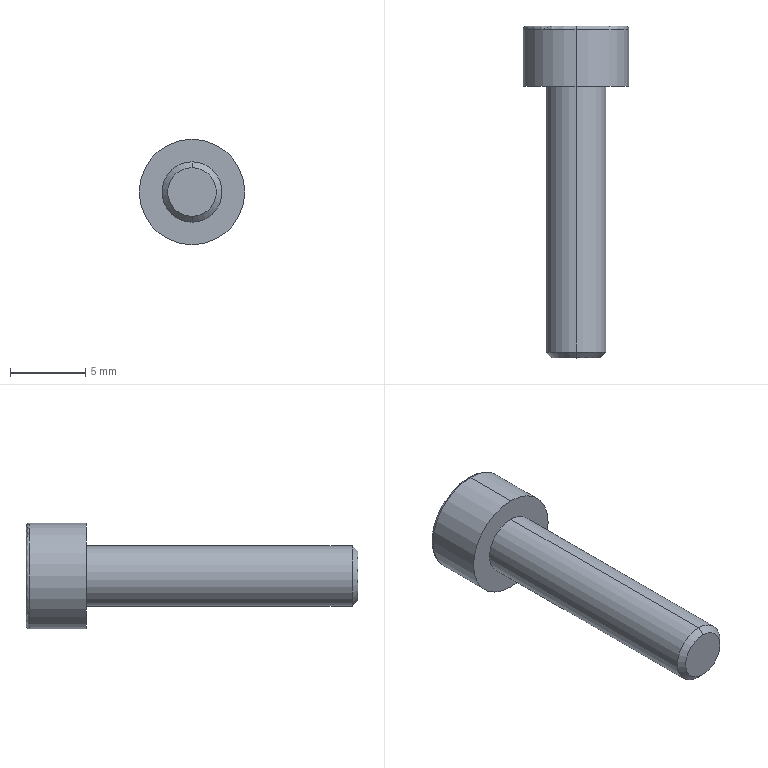Part | SolidWorks | features ICE 2, Chamfer 1, Extrusion 1, Fillet 1, RefAxis 1 | 1 solid | 18 faces | box 7 x 22 x 7 mm | volume 362.728 mm3 | plane 10 | cylinder 4 | cone 2 | torus 2 | commonest cylinder face diameters 4 x2 7 x2
STEP:
#1=CARTESIAN_POINT('',(0.,-18.,-1.61));
#2=VERTEX_POINT('',#1);
#3=CARTESIAN_POINT('',(0.,-18.,1.61));
#4=VERTEX_POINT('',#3);
#5=CARTESIAN_POINT('',(0.,-18.,0.));
#6=DIRECTION('',(0.,-1.,0.));
#7=DIRECTION('',(0.,0.,-1.));
#8=AXIS2_PLACEMENT_3D('',#5,#6,#7);
#9=CIRCLE('',#8,1.61);
#10=EDGE_CURVE('',#2,#4,#9,.T.);
#11=ORIENTED_EDGE('',*,*,#10,.F.);
#12=CARTESIAN_POINT('',(0.,-17.61,-2.));
#13=VERTEX_POINT('',#12);
#14=CARTESIAN_POINT('',(0.,-18.,-1.61));
#15=DIRECTION('',(0.,0.7071,-0.7071));
#16=VECTOR('',#15,1000.);
#17=LINE('',#14,#16);
#18=EDGE_CURVE('',#2,#13,#17,.T.);
#19=ORIENTED_EDGE('',*,*,#18,.T.);
#20=CARTESIAN_POINT('',(0.,-17.61,2.));
#21=VERTEX_POINT('',#20);
#22=CARTESIAN_POINT('',(0.,-17.61,0.));
#23=DIRECTION('',(0.,1.,0.));
#24=DIRECTION('',(0.,0.,-1.));
#25=AXIS2_PLACEMENT_3D('',#22,#23,#24);
#26=CIRCLE('',#25,2.);
#27=EDGE_CURVE('',#21,#13,#26,.T.);
#28=ORIENTED_EDGE('',*,*,#27,.F.);
#29=CARTESIAN_POINT('',(0.,-18.,1.61));
#30=DIRECTION('',(0.,0.7071,0.7071));
#31=VECTOR('',#30,1000.);
#32=LINE('',#29,#31);
#33=EDGE_CURVE('',#4,#21,#32,.T.);
#34=ORIENTED_EDGE('',*,*,#33,.F.);
#35=EDGE_LOOP('',(#11,#19,#28,#34));
#36=FACE_OUTER_BOUND('',#35,.T.);
#37=CARTESIAN_POINT('',(0.,-18.,0.));
#38=DIRECTION('',(0.,1.,0.));
#39=DIRECTION('',(0.,0.,1.));
#40=AXIS2_PLACEMENT_3D('',#37,#38,#39);
#41=CONICAL_SURFACE('',#40,1.61,0.7854);
#42=ADVANCED_FACE('',(#36),#41,.T.);
#43=ORIENTED_EDGE('',*,*,#27,.T.);
#44=CARTESIAN_POINT('',(0.,0.,-2.));
#45=VERTEX_POINT('',#44);
#46=CARTESIAN_POINT('',(0.,-18.,-2.));
#47=DIRECTION('',(0.,1.,0.));
#48=VECTOR('',#47,1000.);
#49=LINE('',#46,#48);
#50=EDGE_CURVE('',#13,#45,#49,.T.);
#51=ORIENTED_EDGE('',*,*,#50,.T.);
#52=CARTESIAN_POINT('',(0.,0.,2.));
#53=VERTEX_POINT('',#52);
#54=CARTESIAN_POINT('',(0.,0.,0.));
#55=DIRECTION('',(0.,-1.,0.));
#56=DIRECTION('',(0.,0.,1.));
#57=AXIS2_PLACEMENT_3D('',#54,#55,#56);
#58=CIRCLE('',#57,2.);
#59=EDGE_CURVE('',#45,#53,#58,.T.);
#60=ORIENTED_EDGE('',*,*,#59,.T.);
#61=CARTESIAN_POINT('',(0.,-18.,2.));
#62=DIRECTION('',(0.,1.,0.));
#63=VECTOR('',#62,1000.);
#64=LINE('',#61,#63);
#65=EDGE_CURVE('',#21,#53,#64,.T.);
#66=ORIENTED_EDGE('',*,*,#65,.F.);
#67=EDGE_LOOP('',(#43,#51,#60,#66));
#68=FACE_OUTER_BOUND('',#67,.T.);
#69=CARTESIAN_POINT('',(0.,-18.,0.));
#70=DIRECTION('',(0.,1.,0.));
#71=DIRECTION('',(0.,0.,1.));
#72=AXIS2_PLACEMENT_3D('',#69,#70,#71);
#73=CYLINDRICAL_SURFACE('',#72,2.);
#74=ADVANCED_FACE('',(#68),#73,.T.);
#75=CARTESIAN_POINT('',(0.,3.8,-3.5));
#76=VERTEX_POINT('',#75);
#77=CARTESIAN_POINT('',(0.,3.8,3.5));
#78=VERTEX_POINT('',#77);
#79=CARTESIAN_POINT('',(0.,3.8,0.));
#80=DIRECTION('',(0.,-1.,0.));
#81=DIRECTION('',(0.,0.,1.));
#82=AXIS2_PLACEMENT_3D('',#79,#80,#81);
#83=CIRCLE('',#82,3.5);
#84=EDGE_CURVE('',#76,#78,#83,.T.);
#85=ORIENTED_EDGE('',*,*,#84,.F.);
#86=CARTESIAN_POINT('',(0.,4.,-3.3));
#87=VERTEX_POINT('',#86);
#88=CARTESIAN_POINT('',(0.,3.8,-3.3));
#89=DIRECTION('',(1.,0.,0.));
#90=DIRECTION('',(0.,0.,-1.));
#91=AXIS2_PLACEMENT_3D('',#88,#89,#90);
#92=CIRCLE('',#91,0.2);
#93=EDGE_CURVE('',#76,#87,#92,.T.);
#94=ORIENTED_EDGE('',*,*,#93,.T.);
#95=CARTESIAN_POINT('',(0.,4.,3.3));
#96=VERTEX_POINT('',#95);
#97=CARTESIAN_POINT('',(0.,4.,0.));
#98=DIRECTION('',(0.,1.,0.));
#99=DIRECTION('',(0.,0.,1.));
#100=AXIS2_PLACEMENT_3D('',#97,#98,#99);
#101=CIRCLE('',#100,3.3);
#102=EDGE_CURVE('',#96,#87,#101,.T.);
#103=ORIENTED_EDGE('',*,*,#102,.F.);
#104=CARTESIAN_POINT('',(0.,3.8,3.3));
#105=DIRECTION('',(-1.,0.,0.));
#106=DIRECTION('',(0.,0.,1.));
#107=AXIS2_PLACEMENT_3D('',#104,#105,#106);
#108=CIRCLE('',#107,0.2);
#109=EDGE_CURVE('',#78,#96,#108,.T.);
#110=ORIENTED_EDGE('',*,*,#109,.F.);
#111=EDGE_LOOP('',(#85,#94,#103,#110));
#112=FACE_OUTER_BOUND('',#111,.T.);
#113=CARTESIAN_POINT('',(0.,3.8,0.));
#114=DIRECTION('',(0.,1.,0.));
#115=DIRECTION('',(0.,0.,1.));
#116=AXIS2_PLACEMENT_3D('',#113,#114,#115);
#117=TOROIDAL_SURFACE('',#116,3.3,0.2);
#118=ADVANCED_FACE('',(#112),#117,.T.);
#119=ORIENTED_EDGE('',*,*,#84,.T.);
#120=CARTESIAN_POINT('',(0.,0.,3.5));
#121=VERTEX_POINT('',#120);
#122=CARTESIAN_POINT('',(0.,4.,3.5));
#123=DIRECTION('',(0.,-1.,0.));
#124=VECTOR('',#123,1000.);
#125=LINE('',#122,#124);
#126=EDGE_CURVE('',#78,#121,#125,.T.);
#127=ORIENTED_EDGE('',*,*,#126,.T.);
#128=CARTESIAN_POINT('',(0.,0.,-3.5));
#129=VERTEX_POINT('',#128);
#130=CARTESIAN_POINT('',(0.,0.,0.));
#131=DIRECTION('',(0.,1.,0.));
#132=DIRECTION('',(0.,0.,1.));
#133=AXIS2_PLACEMENT_3D('',#130,#131,#132);
#134=CIRCLE('',#133,3.5);
#135=EDGE_CURVE('',#121,#129,#134,.T.);
#136=ORIENTED_EDGE('',*,*,#135,.T.);
#137=CARTESIAN_POINT('',(0.,4.,-3.5));
#138=DIRECTION('',(0.,-1.,0.));
#139=VECTOR('',#138,1000.);
#140=LINE('',#137,#139);
#141=EDGE_CURVE('',#76,#129,#140,.T.);
#142=ORIENTED_EDGE('',*,*,#141,.F.);
#143=EDGE_LOOP('',(#119,#127,#136,#142));
#144=FACE_OUTER_BOUND('',#143,.T.);
#145=CARTESIAN_POINT('',(0.,4.,0.));
#146=DIRECTION('',(0.,-1.,0.));
#147=DIRECTION('',(0.,0.,-1.));
#148=AXIS2_PLACEMENT_3D('',#145,#146,#147);
#149=CYLINDRICAL_SURFACE('',#148,3.5);
#150=ADVANCED_FACE('',(#144),#149,.T.);
#151=CARTESIAN_POINT('',(0.,0.,0.));
#152=DIRECTION('',(0.,1.,0.));
#153=DIRECTION('',(0.,0.,1.));
#154=AXIS2_PLACEMENT_3D('',#151,#152,#153);
#155=CIRCLE('',#154,3.5);
#156=EDGE_CURVE('',#129,#121,#155,.T.);
#157=ORIENTED_EDGE('',*,*,#156,.F.);
#158=ORIENTED_EDGE('',*,*,#135,.F.);
#159=EDGE_LOOP('',(#157,#158));
#160=FACE_OUTER_BOUND('',#159,.T.);
#161=CARTESIAN_POINT('',(0.,0.,0.));
#162=DIRECTION('',(0.,-1.,0.));
#163=DIRECTION('',(0.,0.,1.));
#164=AXIS2_PLACEMENT_3D('',#161,#162,#163);
#165=CIRCLE('',#164,2.);
#166=EDGE_CURVE('',#53,#45,#165,.T.);
#167=ORIENTED_EDGE('',*,*,#166,.F.);
#168=ORIENTED_EDGE('',*,*,#59,.F.);
#169=EDGE_LOOP('',(#167,#168));
#170=FACE_BOUND('',#169,.T.);
#171=CARTESIAN_POINT('',(0.,0.,0.));
#172=DIRECTION('',(0.,1.,0.));
#173=DIRECTION('',(0.,0.,1.));
#174=AXIS2_PLACEMENT_3D('',#171,#172,#173);
#175=PLANE('',#174);
#176=ADVANCED_FACE('',(#160,#170),#175,.F.);
#177=ORIENTED_EDGE('',*,*,#126,.F.);
#178=CARTESIAN_POINT('',(0.,3.8,0.));
#179=DIRECTION('',(0.,-1.,0.));
#180=DIRECTION('',(0.,0.,1.));
#181=AXIS2_PLACEMENT_3D('',#178,#179,#180);
#182=CIRCLE('',#181,3.5);
#183=EDGE_CURVE('',#78,#76,#182,.T.);
#184=ORIENTED_EDGE('',*,*,#183,.T.);
#185=ORIENTED_EDGE('',*,*,#141,.T.);
#186=ORIENTED_EDGE('',*,*,#156,.T.);
#187=EDGE_LOOP('',(#177,#184,#185,#186));
#188=FACE_OUTER_BOUND('',#187,.T.);
#189=CARTESIAN_POINT('',(0.,4.,0.));
#190=DIRECTION('',(0.,-1.,0.));
#191=DIRECTION('',(0.,0.,-1.));
#192=AXIS2_PLACEMENT_3D('',#189,#190,#191);
#193=CYLINDRICAL_SURFACE('',#192,3.5);
#194=ADVANCED_FACE('',(#188),#193,.T.);
#195=ORIENTED_EDGE('',*,*,#102,.T.);
#196=CARTESIAN_POINT('',(0.,4.,0.));
#197=DIRECTION('',(0.,1.,0.));
#198=DIRECTION('',(0.,0.,1.));
#199=AXIS2_PLACEMENT_3D('',#196,#197,#198);
#200=CIRCLE('',#199,3.3);
#201=EDGE_CURVE('',#87,#96,#200,.T.);
#202=ORIENTED_EDGE('',*,*,#201,.T.);
#203=EDGE_LOOP('',(#195,#202));
#204=FACE_OUTER_BOUND('',#203,.T.);
#205=CARTESIAN_POINT('',(0.8862,4.,1.535));
#206=VERTEX_POINT('',#205);
#207=CARTESIAN_POINT('',(1.772,4.,0.));
#208=VERTEX_POINT('',#207);
#209=CARTESIAN_POINT('',(0.8862,4.,1.535));
#210=DIRECTION('',(0.5,0.,-0.866));
#211=VECTOR('',#210,1000.);
#212=LINE('',#209,#211);
#213=EDGE_CURVE('',#206,#208,#212,.T.);
#214=ORIENTED_EDGE('',*,*,#213,.F.);
#215=CARTESIAN_POINT('',(-0.8862,4.,1.535));
#216=VERTEX_POINT('',#215);
#217=CARTESIAN_POINT('',(-0.8862,4.,1.535));
#218=DIRECTION('',(1.,0.,0.));
#219=VECTOR('',#218,1000.);
#220=LINE('',#217,#219);
#221=EDGE_CURVE('',#216,#206,#220,.T.);
#222=ORIENTED_EDGE('',*,*,#221,.F.);
#223=CARTESIAN_POINT('',(-1.772,4.,0.));
#224=VERTEX_POINT('',#223);
#225=CARTESIAN_POINT('',(-1.772,4.,0.));
#226=DIRECTION('',(0.5,0.,0.866));
#227=VECTOR('',#226,1000.);
#228=LINE('',#225,#227);
#229=EDGE_CURVE('',#224,#216,#228,.T.);
#230=ORIENTED_EDGE('',*,*,#229,.F.);
#231=CARTESIAN_POINT('',(-0.8862,4.,-1.535));
#232=VERTEX_POINT('',#231);
#233=CARTESIAN_POINT('',(-0.8862,4.,-1.535));
#234=DIRECTION('',(-0.5,0.,0.866));
#235=VECTOR('',#234,1000.);
#236=LINE('',#233,#235);
#237=EDGE_CURVE('',#232,#224,#236,.T.);
#238=ORIENTED_EDGE('',*,*,#237,.F.);
#239=CARTESIAN_POINT('',(0.8862,4.,-1.535));
#240=VERTEX_POINT('',#239);
#241=CARTESIAN_POINT('',(0.8862,4.,-1.535));
#242=DIRECTION('',(-1.,0.,0.));
#243=VECTOR('',#242,1000.);
#244=LINE('',#241,#243);
#245=EDGE_CURVE('',#240,#232,#244,.T.);
#246=ORIENTED_EDGE('',*,*,#245,.F.);
#247=CARTESIAN_POINT('',(1.772,4.,0.));
#248=DIRECTION('',(-0.5,0.,-0.866));
#249=VECTOR('',#248,1000.);
#250=LINE('',#247,#249);
#251=EDGE_CURVE('',#208,#240,#250,.T.);
#252=ORIENTED_EDGE('',*,*,#251,.F.);
#253=EDGE_LOOP('',(#214,#222,#230,#238,#246,#252));
#254=FACE_BOUND('',#253,.T.);
#255=CARTESIAN_POINT('',(0.,4.,0.));
#256=DIRECTION('',(0.,1.,0.));
#257=DIRECTION('',(0.,0.,1.));
#258=AXIS2_PLACEMENT_3D('',#255,#256,#257);
#259=PLANE('',#258);
#260=ADVANCED_FACE('',(#204,#254),#259,.T.);
#261=ORIENTED_EDGE('',*,*,#213,.T.);
#262=CARTESIAN_POINT('',(1.772,2.,0.));
#263=VERTEX_POINT('',#262);
#264=CARTESIAN_POINT('',(1.772,2.,0.));
#265=DIRECTION('',(0.,1.,0.));
#266=VECTOR('',#265,1000.);
#267=LINE('',#264,#266);
#268=EDGE_CURVE('',#263,#208,#267,.T.);
#269=ORIENTED_EDGE('',*,*,#268,.F.);
#270=CARTESIAN_POINT('',(0.8862,2.,1.535));
#271=VERTEX_POINT('',#270);
#272=CARTESIAN_POINT('',(0.8862,2.,1.535));
#273=DIRECTION('',(0.5,0.,-0.866));
#274=VECTOR('',#273,1000.);
#275=LINE('',#272,#274);
#276=EDGE_CURVE('',#271,#263,#275,.T.);
#277=ORIENTED_EDGE('',*,*,#276,.F.);
#278=CARTESIAN_POINT('',(0.8862,2.,1.535));
#279=DIRECTION('',(0.,1.,0.));
#280=VECTOR('',#279,1000.);
#281=LINE('',#278,#280);
#282=EDGE_CURVE('',#271,#206,#281,.T.);
#283=ORIENTED_EDGE('',*,*,#282,.T.);
#284=EDGE_LOOP('',(#261,#269,#277,#283));
#285=FACE_OUTER_BOUND('',#284,.T.);
#286=CARTESIAN_POINT('',(0.8862,2.,1.535));
#287=DIRECTION('',(0.866,0.,0.5));
#288=DIRECTION('',(0.5,0.,-0.866));
#289=AXIS2_PLACEMENT_3D('',#286,#287,#288);
#290=PLANE('',#289);
#291=ADVANCED_FACE('',(#285),#290,.F.);
#292=ORIENTED_EDGE('',*,*,#221,.T.);
#293=ORIENTED_EDGE('',*,*,#282,.F.);
#294=CARTESIAN_POINT('',(-0.8862,2.,1.535));
#295=VERTEX_POINT('',#294);
#296=CARTESIAN_POINT('',(-0.8862,2.,1.535));
#297=DIRECTION('',(1.,0.,0.));
#298=VECTOR('',#297,1000.);
#299=LINE('',#296,#298);
#300=EDGE_CURVE('',#295,#271,#299,.T.);
#301=ORIENTED_EDGE('',*,*,#300,.F.);
#302=CARTESIAN_POINT('',(-0.8862,2.,1.535));
#303=DIRECTION('',(0.,1.,0.));
#304=VECTOR('',#303,1000.);
#305=LINE('',#302,#304);
#306=EDGE_CURVE('',#295,#216,#305,.T.);
#307=ORIENTED_EDGE('',*,*,#306,.T.);
#308=EDGE_LOOP('',(#292,#293,#301,#307));
#309=FACE_OUTER_BOUND('',#308,.T.);
#310=CARTESIAN_POINT('',(-0.8862,2.,1.535));
#311=DIRECTION('',(0.,0.,1.));
#312=DIRECTION('',(1.,0.,0.));
#313=AXIS2_PLACEMENT_3D('',#310,#311,#312);
#314=PLANE('',#313);
#315=ADVANCED_FACE('',(#309),#314,.F.);
#316=ORIENTED_EDGE('',*,*,#229,.T.);
#317=ORIENTED_EDGE('',*,*,#306,.F.);
#318=CARTESIAN_POINT('',(-1.772,2.,0.));
#319=VERTEX_POINT('',#318);
#320=CARTESIAN_POINT('',(-1.772,2.,0.));
#321=DIRECTION('',(0.5,0.,0.866));
#322=VECTOR('',#321,1000.);
#323=LINE('',#320,#322);
#324=EDGE_CURVE('',#319,#295,#323,.T.);
#325=ORIENTED_EDGE('',*,*,#324,.F.);
#326=CARTESIAN_POINT('',(-1.772,2.,0.));
#327=DIRECTION('',(0.,1.,0.));
#328=VECTOR('',#327,1000.);
#329=LINE('',#326,#328);
#330=EDGE_CURVE('',#319,#224,#329,.T.);
#331=ORIENTED_EDGE('',*,*,#330,.T.);
#332=EDGE_LOOP('',(#316,#317,#325,#331));
#333=FACE_OUTER_BOUND('',#332,.T.);
#334=CARTESIAN_POINT('',(-1.772,2.,0.));
#335=DIRECTION('',(-0.866,0.,0.5));
#336=DIRECTION('',(0.5,0.,0.866));
#337=AXIS2_PLACEMENT_3D('',#334,#335,#336);
#338=PLANE('',#337);
#339=ADVANCED_FACE('',(#333),#338,.F.);
#340=ORIENTED_EDGE('',*,*,#237,.T.);
#341=ORIENTED_EDGE('',*,*,#330,.F.);
#342=CARTESIAN_POINT('',(-0.8862,2.,-1.535));
#343=VERTEX_POINT('',#342);
#344=CARTESIAN_POINT('',(-0.8862,2.,-1.535));
#345=DIRECTION('',(-0.5,0.,0.866));
#346=VECTOR('',#345,1000.);
#347=LINE('',#344,#346);
#348=EDGE_CURVE('',#343,#319,#347,.T.);
#349=ORIENTED_EDGE('',*,*,#348,.F.);
#350=CARTESIAN_POINT('',(-0.8862,2.,-1.535));
#351=DIRECTION('',(0.,1.,0.));
#352=VECTOR('',#351,1000.);
#353=LINE('',#350,#352);
#354=EDGE_CURVE('',#343,#232,#353,.T.);
#355=ORIENTED_EDGE('',*,*,#354,.T.);
#356=EDGE_LOOP('',(#340,#341,#349,#355));
#357=FACE_OUTER_BOUND('',#356,.T.);
#358=CARTESIAN_POINT('',(-0.8862,2.,-1.535));
#359=DIRECTION('',(-0.866,0.,-0.5));
#360=DIRECTION('',(-0.5,0.,0.866));
#361=AXIS2_PLACEMENT_3D('',#358,#359,#360);
#362=PLANE('',#361);
#363=ADVANCED_FACE('',(#357),#362,.F.);
#364=ORIENTED_EDGE('',*,*,#245,.T.);
#365=ORIENTED_EDGE('',*,*,#354,.F.);
#366=CARTESIAN_POINT('',(0.8862,2.,-1.535));
#367=VERTEX_POINT('',#366);
#368=CARTESIAN_POINT('',(0.8862,2.,-1.535));
#369=DIRECTION('',(-1.,0.,0.));
#370=VECTOR('',#369,1000.);
#371=LINE('',#368,#370);
#372=EDGE_CURVE('',#367,#343,#371,.T.);
#373=ORIENTED_EDGE('',*,*,#372,.F.);
#374=CARTESIAN_POINT('',(0.8862,2.,-1.535));
#375=DIRECTION('',(0.,1.,0.));
#376=VECTOR('',#375,1000.);
#377=LINE('',#374,#376);
#378=EDGE_CURVE('',#367,#240,#377,.T.);
#379=ORIENTED_EDGE('',*,*,#378,.T.);
#380=EDGE_LOOP('',(#364,#365,#373,#379));
#381=FACE_OUTER_BOUND('',#380,.T.);
#382=CARTESIAN_POINT('',(0.8862,2.,-1.535));
#383=DIRECTION('',(0.,0.,-1.));
#384=DIRECTION('',(-1.,0.,0.));
#385=AXIS2_PLACEMENT_3D('',#382,#383,#384);
#386=PLANE('',#385);
#387=ADVANCED_FACE('',(#381),#386,.F.);
#388=ORIENTED_EDGE('',*,*,#251,.T.);
#389=ORIENTED_EDGE('',*,*,#378,.F.);
#390=CARTESIAN_POINT('',(1.772,2.,0.));
#391=DIRECTION('',(-0.5,0.,-0.866));
#392=VECTOR('',#391,1000.);
#393=LINE('',#390,#392);
#394=EDGE_CURVE('',#263,#367,#393,.T.);
#395=ORIENTED_EDGE('',*,*,#394,.F.);
#396=ORIENTED_EDGE('',*,*,#268,.T.);
#397=EDGE_LOOP('',(#388,#389,#395,#396));
#398=FACE_OUTER_BOUND('',#397,.T.);
#399=CARTESIAN_POINT('',(1.772,2.,0.));
#400=DIRECTION('',(0.866,0.,-0.5));
#401=DIRECTION('',(-0.5,0.,-0.866));
#402=AXIS2_PLACEMENT_3D('',#399,#400,#401);
#403=PLANE('',#402);
#404=ADVANCED_FACE('',(#398),#403,.F.);
#405=ORIENTED_EDGE('',*,*,#276,.T.);
#406=ORIENTED_EDGE('',*,*,#394,.T.);
#407=ORIENTED_EDGE('',*,*,#372,.T.);
#408=ORIENTED_EDGE('',*,*,#348,.T.);
#409=ORIENTED_EDGE('',*,*,#324,.T.);
#410=ORIENTED_EDGE('',*,*,#300,.T.);
#411=EDGE_LOOP('',(#405,#406,#407,#408,#409,#410));
#412=FACE_OUTER_BOUND('',#411,.T.);
#413=CARTESIAN_POINT('',(0.,2.,0.));
#414=DIRECTION('',(0.,1.,0.));
#415=DIRECTION('',(0.,0.,1.));
#416=AXIS2_PLACEMENT_3D('',#413,#414,#415);
#417=PLANE('',#416);
#418=ADVANCED_FACE('',(#412),#417,.T.);
#419=ORIENTED_EDGE('',*,*,#93,.F.);
#420=ORIENTED_EDGE('',*,*,#183,.F.);
#421=ORIENTED_EDGE('',*,*,#109,.T.);
#422=ORIENTED_EDGE('',*,*,#201,.F.);
#423=EDGE_LOOP('',(#419,#420,#421,#422));
#424=FACE_OUTER_BOUND('',#423,.T.);
#425=CARTESIAN_POINT('',(0.,3.8,0.));
#426=DIRECTION('',(0.,1.,0.));
#427=DIRECTION('',(0.,0.,1.));
#428=AXIS2_PLACEMENT_3D('',#425,#426,#427);
#429=TOROIDAL_SURFACE('',#428,3.3,0.2);
#430=ADVANCED_FACE('',(#424),#429,.T.);
#431=ORIENTED_EDGE('',*,*,#50,.F.);
#432=CARTESIAN_POINT('',(0.,-17.61,0.));
#433=DIRECTION('',(0.,1.,0.));
#434=DIRECTION('',(0.,0.,-1.));
#435=AXIS2_PLACEMENT_3D('',#432,#433,#434);
#436=CIRCLE('',#435,2.);
#437=EDGE_CURVE('',#13,#21,#436,.T.);
#438=ORIENTED_EDGE('',*,*,#437,.T.);
#439=ORIENTED_EDGE('',*,*,#65,.T.);
#440=ORIENTED_EDGE('',*,*,#166,.T.);
#441=EDGE_LOOP('',(#431,#438,#439,#440));
#442=FACE_OUTER_BOUND('',#441,.T.);
#443=CARTESIAN_POINT('',(0.,-18.,0.));
#444=DIRECTION('',(0.,1.,0.));
#445=DIRECTION('',(0.,0.,1.));
#446=AXIS2_PLACEMENT_3D('',#443,#444,#445);
#447=CYLINDRICAL_SURFACE('',#446,2.);
#448=ADVANCED_FACE('',(#442),#447,.T.);
#449=CARTESIAN_POINT('',(0.,-18.,0.));
#450=DIRECTION('',(0.,-1.,0.));
#451=DIRECTION('',(0.,0.,-1.));
#452=AXIS2_PLACEMENT_3D('',#449,#450,#451);
#453=CIRCLE('',#452,1.61);
#454=EDGE_CURVE('',#4,#2,#453,.T.);
#455=ORIENTED_EDGE('',*,*,#454,.T.);
#456=ORIENTED_EDGE('',*,*,#10,.T.);
#457=EDGE_LOOP('',(#455,#456));
#458=FACE_OUTER_BOUND('',#457,.T.);
#459=CARTESIAN_POINT('',(0.,-18.,0.));
#460=DIRECTION('',(0.,-1.,0.));
#461=DIRECTION('',(0.,0.,-1.));
#462=AXIS2_PLACEMENT_3D('',#459,#460,#461);
#463=PLANE('',#462);
#464=ADVANCED_FACE('',(#458),#463,.T.);
#465=ORIENTED_EDGE('',*,*,#18,.F.);
#466=ORIENTED_EDGE('',*,*,#454,.F.);
#467=ORIENTED_EDGE('',*,*,#33,.T.);
#468=ORIENTED_EDGE('',*,*,#437,.F.);
#469=EDGE_LOOP('',(#465,#466,#467,#468));
#470=FACE_OUTER_BOUND('',#469,.T.);
#471=CARTESIAN_POINT('',(0.,-18.,0.));
#472=DIRECTION('',(0.,1.,0.));
#473=DIRECTION('',(0.,0.,1.));
#474=AXIS2_PLACEMENT_3D('',#471,#472,#473);
#475=CONICAL_SURFACE('',#474,1.61,0.7854);
#476=ADVANCED_FACE('',(#470),#475,.T.);
#477=CLOSED_SHELL('',(#42,#74,#118,#150,#176,#194,#260,#291,#315,#339,#363,#387,#404,#418,#430,#448,#464,#476));
#478=MANIFOLD_SOLID_BREP('',#477);
#479=CARTESIAN_POINT('',(0.,0.,0.));
#480=DIRECTION('',(0.,0.,1.));
#481=DIRECTION('',(1.,0.,0.));
#482=AXIS2_PLACEMENT_3D('',#479,#480,#481);
#483=(LENGTH_UNIT()NAMED_UNIT(*)SI_UNIT(.MILLI.,.METRE.));
#484=UNCERTAINTY_MEASURE_WITH_UNIT(LENGTH_MEASURE(0.00001),#483,'','');
#485=(NAMED_UNIT(*)PLANE_ANGLE_UNIT()SI_UNIT($,.RADIAN.));
#486=(NAMED_UNIT(*)SI_UNIT($,.STERADIAN.)SOLID_ANGLE_UNIT());
#487=(GEOMETRIC_REPRESENTATION_CONTEXT(3)GLOBAL_UNCERTAINTY_ASSIGNED_CONTEXT((#484))GLOBAL_UNIT_ASSIGNED_CONTEXT((#483,#485,#486))REPRESENTATION_CONTEXT('',''));
#488=ADVANCED_BREP_SHAPE_REPRESENTATION('',(#478,#482),#487);